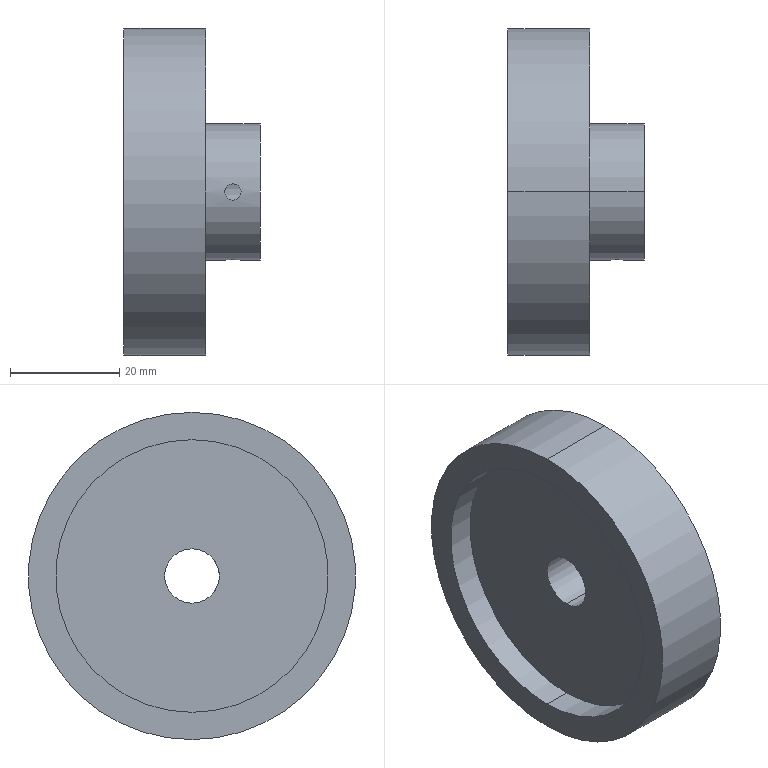Part | STEP file | Handle | 1 solid | 16 faces | box 25 x 60 x 60 mm | volume 35825 mm3 | cylinder 12 | plane 4 | commonest cylinder face diameters 3 x4 10 x2 25 x2 50 x2 60 x2